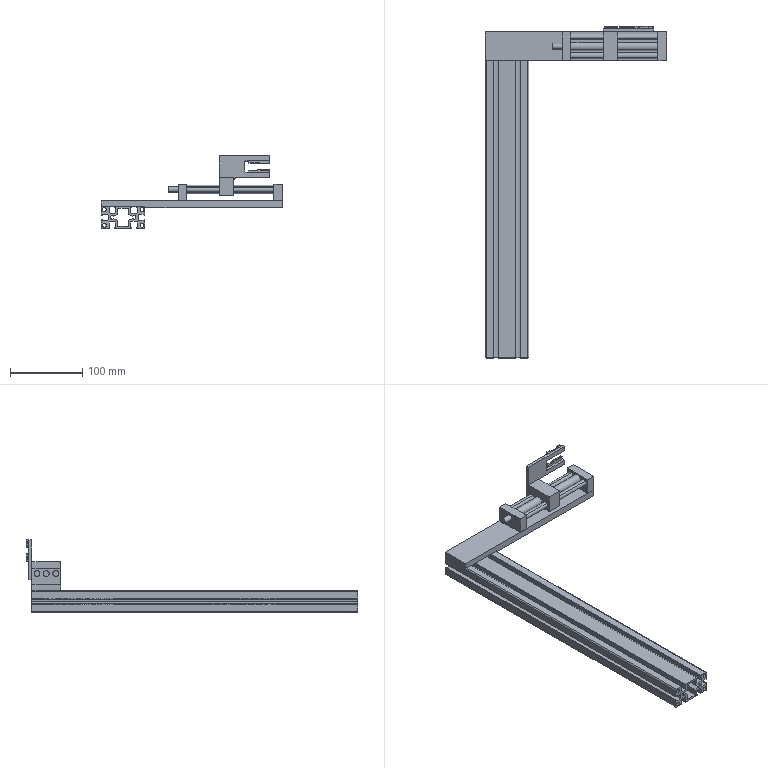Part | SolidWorks | 13 solids | 311 faces | box 250 x 458 x 100.154 mm | volume 518648 mm3 | plane 218 | cylinder 93 | commonest cylinder face diameters 8 x24 2.1 x10 3.6 x10 2.2 x8 5.3 x8 24 x7